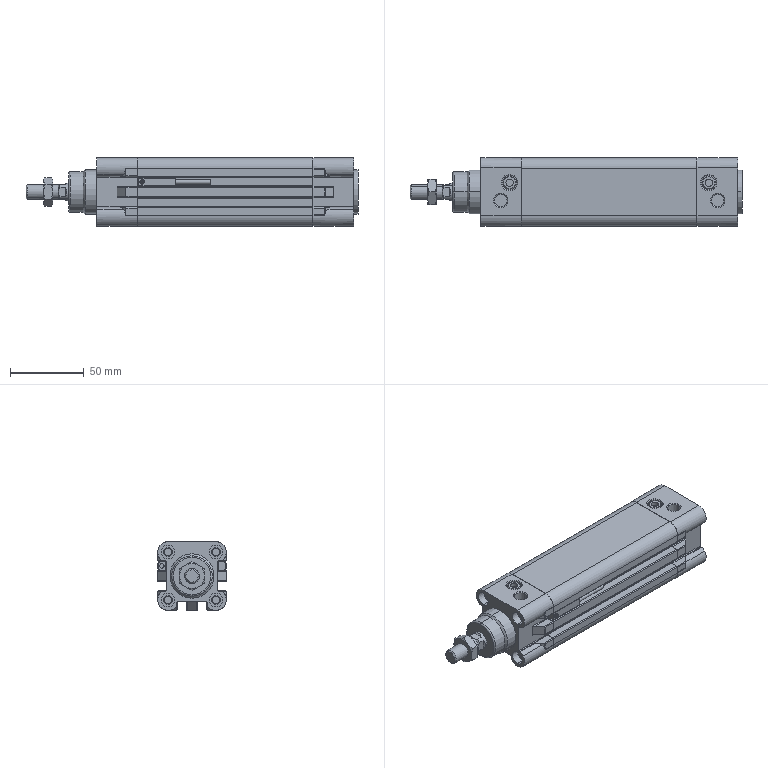Part | 5 solids | 504 faces | box 225 x 47.1 x 46.5 mm | volume 271429 mm3 | plane 229 | cylinder 206 | cone 67 | torus 2 | commonest cylinder face diameters 1 x90 4.917 x16 9.4 x16 8 x12 14 x10 15 x10